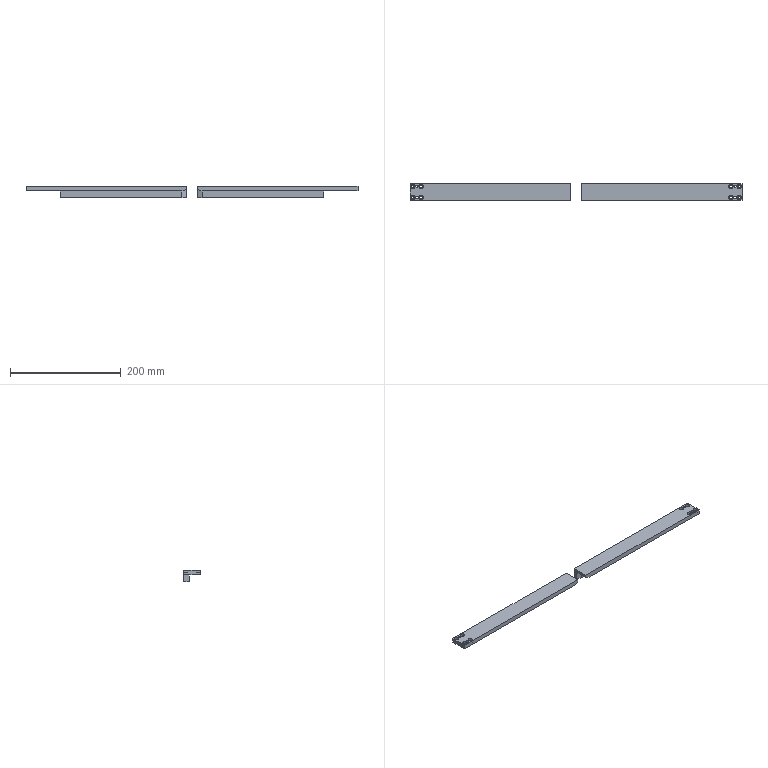NC program | NX | posted with a generic post | part box 600 x 30 x 20 mm
Lines 415 to 1233 of 3385:
(ZLEVEL_PROFILE_COPY_1_COPY_1 , TOOL : D3)
N792 T20 M6
N794 G54
N796 G17 G0 G90 X132.15 Y9.714 S7000 M3
N798 G43 Z30. H20
N800 Z1.
N802 G94 G1 X132.179 Y9.67 Z0.997 F1000.
N804 X132.383 Y9.555 Z0.985
N806 X132.617 Z0.973
N808 X132.821 Y9.67 Z0.96
N810 X132.927 Y9.829 Z0.95
N812 X132.951 Y10.089 Z0.937
N814 X132.83 Y10.321 Z0.923
N816 X132.671 Y10.427 Z0.913
N818 X132.595 Y10.45 Z0.909
N820 X132.405 Z0.899
N822 X132.179 Y10.33 Z0.885
N824 X132.073 Y10.171 Z0.875
N826 X132.04 Y10. Z0.866
N828 X132.073 Y9.829 Z0.857
N830 X132.179 Y9.67 Z0.847
N832 X132.383 Y9.555 Z0.835
N834 X132.617 Z0.823
N836 X132.821 Y9.67 Z0.81
N838 X132.927 Y9.829 Z0.8
N840 X132.951 Y10.089 Z0.787
N842 X132.83 Y10.321 Z0.773
N844 X132.671 Y10.427 Z0.763
N846 X132.595 Y10.45 Z0.759
N848 X132.405 Z0.749
N850 X132.179 Y10.33 Z0.735
N852 X132.073 Y10.171 Z0.725
N854 X132.04 Y10. Z0.716
N856 X132.073 Y9.829 Z0.707
N858 X132.179 Y9.67 Z0.697
N860 X132.383 Y9.555 Z0.685
N862 X132.617 Z0.673
N864 X132.821 Y9.67 Z0.66
N866 X132.927 Y9.829 Z0.65
N868 X132.951 Y10.089 Z0.637
N870 X132.83 Y10.321 Z0.623
N872 X132.671 Y10.427 Z0.613
N874 X132.595 Y10.45 Z0.609
N876 X132.405 Z0.599
N878 X132.179 Y10.33 Z0.585
N880 X132.073 Y10.171 Z0.575
N882 X132.04 Y10. Z0.566
N884 X132.073 Y9.829 Z0.557
N886 X132.179 Y9.67 Z0.547
N888 X132.383 Y9.555 Z0.535
N890 X132.617 Z0.523
N892 X132.821 Y9.67 Z0.51
N894 X132.927 Y9.829 Z0.5
N896 X132.951 Y10.089 Z0.487
N898 X132.83 Y10.321 Z0.473
N900 X132.671 Y10.427 Z0.463
N902 X132.595 Y10.45 Z0.459
N904 X132.405 Z0.449
N906 X132.179 Y10.33 Z0.435
N908 X132.073 Y10.171 Z0.425
N910 X132.04 Y10. Z0.416
N912 X132.073 Y9.829 Z0.407
N914 X132.179 Y9.67 Z0.397
N916 X132.383 Y9.555 Z0.385
N918 X132.617 Z0.373
N920 X132.821 Y9.67 Z0.36
N922 X132.927 Y9.829 Z0.35
N924 X132.951 Y10.089 Z0.337
N926 X132.83 Y10.321 Z0.323
N928 X132.671 Y10.427 Z0.313
N930 X132.595 Y10.45 Z0.309
N932 X132.405 Z0.299
N934 X132.179 Y10.33 Z0.285
N936 X132.073 Y10.171 Z0.275
N938 X132.04 Y10. Z0.266
N940 X132.073 Y9.829 Z0.257
N942 X132.179 Y9.67 Z0.247
N944 X132.383 Y9.555 Z0.235
N946 X132.617 Z0.223
N948 X132.821 Y9.67 Z0.21
N950 X132.927 Y9.829 Z0.2
N952 X132.951 Y10.089 Z0.187
N954 X132.83 Y10.321 Z0.173
N956 X132.671 Y10.427 Z0.163
N958 X132.595 Y10.45 Z0.159
N960 X132.405 Z0.149
N962 X132.179 Y10.33 Z0.135
N964 X132.073 Y10.171 Z0.125
N966 X132.04 Y10. Z0.116
N968 X132.073 Y9.829 Z0.107
N970 X132.179 Y9.67 Z0.097
N972 X132.383 Y9.555 Z0.085
N974 X132.617 Z0.073
N976 X132.821 Y9.67 Z0.06
N978 X132.927 Y9.829 Z0.05
N980 X132.951 Y10.089 Z0.037
N982 X132.83 Y10.321 Z0.023
N984 X132.671 Y10.427 Z0.013
N986 X132.595 Y10.45 Z0.009
N988 X132.405 Z-0.001
N990 X132.179 Y10.33 Z-0.015
N992 X132.073 Y10.171 Z-0.025
N994 X132.04 Y10. Z-0.034
N996 X132.073 Y9.829 Z-0.043
N998 X132.179 Y9.67 Z-0.053
N1000 X132.383 Y9.555 Z-0.065
N1002 X132.617 Z-0.077
N1004 X132.821 Y9.67 Z-0.09
N1006 X132.927 Y9.829 Z-0.1
N1008 X132.951 Y10.089 Z-0.113
N1010 X132.83 Y10.321 Z-0.127
N1012 X132.671 Y10.427 Z-0.137
N1014 X132.595 Y10.45 Z-0.141
N1016 X132.405 Z-0.151
N1018 X132.179 Y10.33 Z-0.165
N1020 X132.073 Y10.171 Z-0.175
N1022 X132.04 Y10. Z-0.184
N1024 X132.073 Y9.829 Z-0.193
N1026 X132.179 Y9.67 Z-0.203
N1028 X132.383 Y9.555 Z-0.215
N1030 X132.617 Z-0.227
N1032 X132.821 Y9.67 Z-0.24
N1034 X132.927 Y9.829 Z-0.25
N1036 X132.951 Y10.089 Z-0.263
N1038 X132.83 Y10.321 Z-0.277
N1040 X132.671 Y10.427 Z-0.287
N1042 X132.595 Y10.45 Z-0.291
N1044 X132.5 Z-0.296
N1046 G3 X132.05 Y10. R0.45 F1300.
N1048 X132.5 Y10.45 R-0.45
N1050 G1 X132.443 Y10.439 Z-0.305
N1052 X132.387 Y10.427 Z-0.313
N1054 X132.331 Y10.411 Z-0.321
N1056 X132.279 Y10.383 Z-0.329
N1058 X132.23 Y10.351 Z-0.337
N1060 X132.186 Y10.314 Z-0.346
N1062 X132.149 Y10.27 Z-0.354
N1064 X132.117 Y10.221 Z-0.362
N1066 X132.089 Y10.169 Z-0.37
N1068 X132.073 Y10.113 Z-0.379
N1070 X132.054 Y10.059 Z-0.387
N1072 X132.05 Y10. Z-0.395
N1074 X132.054 Y9.941 Z-0.403
N1076 X132.065 Y9.884 Z-0.412
N1078 X132.084 Y9.828 Z-0.42
N1080 X132.11 Y9.775 Z-0.428
N1082 X132.149 Y9.732 Z-0.436
N1084 X132.185 Y9.687 Z-0.444
N1086 X132.23 Y9.65 Z-0.453
N1088 X132.279 Y9.617 Z-0.461
N1090 X132.331 Y9.59 Z-0.469
N1092 X132.386 Y9.573 Z-0.477
N1094 X132.442 Y9.561 Z-0.486
N1096 X132.5 Y9.556 Z-0.494
N1098 X132.558 Y9.561 Z-0.502
N1100 X132.614 Y9.573 Z-0.51
N1102 X132.669 Y9.59 Z-0.519
N1104 X132.721 Y9.617 Z-0.527
N1106 X132.77 Y9.649 Z-0.535
N1108 X132.814 Y9.686 Z-0.543
N1110 X132.851 Y9.73 Z-0.551
N1112 X132.883 Y9.779 Z-0.56
N1114 X132.911 Y9.831 Z-0.568
N1116 X132.927 Y9.887 Z-0.576
N1118 X132.939 Y9.943 Z-0.584
N1120 X132.95 Y10. Z-0.593
N1122 G3 X132.5 Y10.45 R0.45
N1124 G1 X132.443 Y10.439 Z-0.601
N1126 X132.387 Y10.427 Z-0.609
N1128 X132.331 Y10.411 Z-0.617
N1130 X132.279 Y10.383 Z-0.626
N1132 X132.23 Y10.351 Z-0.634
N1134 X132.186 Y10.314 Z-0.642
N1136 X132.149 Y10.27 Z-0.65
N1138 X132.117 Y10.221 Z-0.658
N1140 X132.089 Y10.169 Z-0.667
N1142 X132.073 Y10.113 Z-0.675
N1144 X132.054 Y10.059 Z-0.683
N1146 X132.05 Y10. Z-0.691
N1148 X132.054 Y9.941 Z-0.7
N1150 X132.065 Y9.884 Z-0.708
N1152 X132.084 Y9.828 Z-0.716
N1154 X132.11 Y9.775 Z-0.724
N1156 X132.149 Y9.732 Z-0.733
N1158 X132.185 Y9.687 Z-0.741
N1160 X132.23 Y9.65 Z-0.749
N1162 X132.279 Y9.617 Z-0.757
N1164 X132.331 Y9.59 Z-0.765
N1166 X132.386 Y9.573 Z-0.774
N1168 X132.442 Y9.561 Z-0.782
N1170 X132.5 Y9.556 Z-0.79
N1172 X132.558 Y9.561 Z-0.798
N1174 X132.614 Y9.573 Z-0.807
N1176 X132.669 Y9.59 Z-0.815
N1178 X132.721 Y9.617 Z-0.823
N1180 X132.77 Y9.649 Z-0.831
N1182 X132.814 Y9.686 Z-0.84
N1184 X132.851 Y9.73 Z-0.848
N1186 X132.883 Y9.779 Z-0.856
N1188 X132.911 Y9.831 Z-0.864
N1190 X132.927 Y9.887 Z-0.872
N1192 X132.939 Y9.943 Z-0.881
N1194 X132.95 Y10. Z-0.889
N1196 G3 X132.5 Y10.45 R0.45
N1198 G1 X132.443 Y10.439 Z-0.897
N1200 X132.387 Y10.427 Z-0.905
N1202 X132.331 Y10.411 Z-0.914
N1204 X132.279 Y10.383 Z-0.922
N1206 X132.23 Y10.351 Z-0.93
N1208 X132.186 Y10.314 Z-0.938
N1210 X132.149 Y10.27 Z-0.947
N1212 X132.117 Y10.221 Z-0.955
N1214 X132.089 Y10.169 Z-0.963
N1216 X132.073 Y10.113 Z-0.971
N1218 X132.054 Y10.059 Z-0.979
N1220 X132.05 Y10. Z-0.988
N1222 X132.054 Y9.941 Z-0.996
N1224 X132.065 Y9.884 Z-1.004
N1226 X132.084 Y9.828 Z-1.012
N1228 X132.11 Y9.775 Z-1.021
N1230 X132.149 Y9.732 Z-1.029
N1232 X132.185 Y9.687 Z-1.037
N1234 X132.23 Y9.65 Z-1.045
N1236 X132.279 Y9.617 Z-1.053
N1238 X132.331 Y9.59 Z-1.062
N1240 X132.386 Y9.573 Z-1.07
N1242 X132.442 Y9.561 Z-1.078
N1244 X132.5 Y9.556 Z-1.086
N1246 X132.558 Y9.561 Z-1.095
N1248 X132.614 Y9.573 Z-1.103
N1250 X132.669 Y9.59 Z-1.111
N1252 X132.721 Y9.617 Z-1.119
N1254 X132.77 Y9.649 Z-1.128
N1256 X132.814 Y9.686 Z-1.136
N1258 X132.851 Y9.73 Z-1.144
N1260 X132.883 Y9.779 Z-1.152
N1262 X132.911 Y9.831 Z-1.16
N1264 X132.927 Y9.887 Z-1.169
N1266 X132.939 Y9.943 Z-1.177
N1268 X132.95 Y10. Z-1.185
N1270 G3 X132.5 Y10.45 R0.45
N1272 G1 X132.443 Y10.439 Z-1.193
N1274 X132.387 Y10.427 Z-1.202
N1276 X132.331 Y10.411 Z-1.21
N1278 X132.279 Y10.383 Z-1.218
N1280 X132.23 Y10.351 Z-1.226
N1282 X132.186 Y10.314 Z-1.235
N1284 X132.149 Y10.27 Z-1.243
N1286 X132.117 Y10.221 Z-1.251
N1288 X132.089 Y10.169 Z-1.259
N1290 X132.073 Y10.113 Z-1.267
N1292 X132.054 Y10.059 Z-1.276
N1294 X132.05 Y10. Z-1.284
N1296 X132.054 Y9.941 Z-1.292
N1298 X132.065 Y9.884 Z-1.3
N1300 X132.084 Y9.828 Z-1.309
N1302 X132.11 Y9.775 Z-1.317
N1304 X132.149 Y9.732 Z-1.325
N1306 X132.185 Y9.687 Z-1.333
N1308 X132.23 Y9.65 Z-1.342
N1310 X132.279 Y9.617 Z-1.35
N1312 X132.331 Y9.59 Z-1.358
N1314 X132.386 Y9.573 Z-1.366
N1316 X132.442 Y9.561 Z-1.374
N1318 X132.5 Y9.556 Z-1.383
N1320 X132.558 Y9.561 Z-1.391
N1322 X132.614 Y9.573 Z-1.399
N1324 X132.669 Y9.59 Z-1.407
N1326 X132.721 Y9.617 Z-1.416
N1328 X132.77 Y9.649 Z-1.424
N1330 X132.814 Y9.686 Z-1.432
N1332 X132.851 Y9.73 Z-1.44
N1334 X132.883 Y9.779 Z-1.449
N1336 X132.911 Y9.831 Z-1.457
N1338 X132.927 Y9.887 Z-1.465
N1340 X132.939 Y9.943 Z-1.473
N1342 X132.95 Y10. Z-1.481
N1344 G3 X132.5 Y10.45 R0.45
N1346 G1 X132.443 Y10.439 Z-1.49
N1348 X132.387 Y10.427 Z-1.498
N1350 X132.331 Y10.411 Z-1.506
N1352 X132.279 Y10.383 Z-1.514
N1354 X132.23 Y10.351 Z-1.523
N1356 X132.186 Y10.314 Z-1.531
N1358 X132.149 Y10.27 Z-1.539
N1360 X132.117 Y10.221 Z-1.547
N1362 X132.089 Y10.169 Z-1.556
N1364 X132.073 Y10.113 Z-1.564
N1366 X132.054 Y10.059 Z-1.572
N1368 X132.05 Y10. Z-1.58
N1370 X132.054 Y9.941 Z-1.588
N1372 X132.065 Y9.884 Z-1.597
N1374 X132.084 Y9.828 Z-1.605
N1376 X132.11 Y9.775 Z-1.613
N1378 X132.149 Y9.732 Z-1.621
N1380 X132.185 Y9.687 Z-1.63
N1382 X132.23 Y9.65 Z-1.638
N1384 X132.279 Y9.617 Z-1.646
N1386 X132.331 Y9.59 Z-1.654
N1388 X132.386 Y9.573 Z-1.663
N1390 X132.442 Y9.561 Z-1.671
N1392 X132.5 Y9.556 Z-1.679
N1394 X132.558 Y9.561 Z-1.687
N1396 X132.614 Y9.573 Z-1.695
N1398 X132.669 Y9.59 Z-1.704
N1400 X132.721 Y9.617 Z-1.712
N1402 X132.77 Y9.649 Z-1.72
N1404 X132.814 Y9.686 Z-1.728
N1406 X132.851 Y9.73 Z-1.737
N1408 X132.883 Y9.779 Z-1.745
N1410 X132.911 Y9.831 Z-1.753
N1412 X132.927 Y9.887 Z-1.761
N1414 X132.939 Y9.943 Z-1.77
N1416 X132.95 Y10. Z-1.778
N1418 G3 X132.5 Y10.45 R0.45
N1420 G1 X132.443 Y10.439 Z-1.786
N1422 X132.387 Y10.427 Z-1.794
N1424 X132.331 Y10.411 Z-1.802
N1426 X132.279 Y10.383 Z-1.811
N1428 X132.23 Y10.351 Z-1.819
N1430 X132.186 Y10.314 Z-1.827
N1432 X132.149 Y10.27 Z-1.835
N1434 X132.117 Y10.221 Z-1.844
N1436 X132.089 Y10.169 Z-1.852
N1438 X132.073 Y10.113 Z-1.86
N1440 X132.054 Y10.059 Z-1.868
N1442 X132.05 Y10. Z-1.877
N1444 X132.054 Y9.941 Z-1.885
N1446 X132.065 Y9.884 Z-1.893
N1448 X132.084 Y9.828 Z-1.901
N1450 X132.11 Y9.775 Z-1.909
N1452 X132.149 Y9.732 Z-1.918
N1454 X132.185 Y9.687 Z-1.926
N1456 X132.23 Y9.65 Z-1.934
N1458 X132.279 Y9.617 Z-1.942
N1460 X132.331 Y9.59 Z-1.951
N1462 X132.386 Y9.573 Z-1.959
N1464 X132.442 Y9.561 Z-1.967
N1466 X132.5 Y9.556 Z-1.975
N1468 X132.558 Y9.561 Z-1.984
N1470 X132.614 Y9.573 Z-1.992
N1472 X132.669 Y9.59 Z-2.
N1474 X132.721 Y9.617 Z-2.008
N1476 X132.77 Y9.649 Z-2.016
N1478 X132.814 Y9.686 Z-2.025
N1480 X132.851 Y9.73 Z-2.033
N1482 X132.883 Y9.779 Z-2.041
N1484 X132.911 Y9.831 Z-2.049
N1486 X132.927 Y9.887 Z-2.058
N1488 X132.939 Y9.943 Z-2.066
N1490 X132.95 Y10. Z-2.074
N1492 G3 X132.5 Y10.45 R0.45
N1494 G1 X132.443 Y10.439 Z-2.082
N1496 X132.387 Y10.427 Z-2.091
N1498 X132.331 Y10.411 Z-2.099
N1500 X132.279 Y10.383 Z-2.107
N1502 X132.23 Y10.351 Z-2.115
N1504 X132.186 Y10.314 Z-2.123
N1506 X132.149 Y10.27 Z-2.132
N1508 X132.117 Y10.221 Z-2.14
N1510 X132.089 Y10.169 Z-2.148
N1512 X132.073 Y10.113 Z-2.156
N1514 X132.054 Y10.059 Z-2.165
N1516 X132.05 Y10. Z-2.173
N1518 X132.054 Y9.941 Z-2.181
N1520 X132.065 Y9.884 Z-2.189
N1522 X132.084 Y9.828 Z-2.198
N1524 X132.11 Y9.775 Z-2.206
N1526 X132.149 Y9.732 Z-2.214
N1528 X132.185 Y9.687 Z-2.222
N1530 X132.23 Y9.65 Z-2.23
N1532 X132.279 Y9.617 Z-2.239
N1534 X132.331 Y9.59 Z-2.247
N1536 X132.386 Y9.573 Z-2.255
N1538 X132.442 Y9.561 Z-2.263
N1540 X132.5 Y9.556 Z-2.272
N1542 X132.558 Y9.561 Z-2.28
N1544 X132.614 Y9.573 Z-2.288
N1546 X132.669 Y9.59 Z-2.296
N1548 X132.721 Y9.617 Z-2.305
N1550 X132.77 Y9.649 Z-2.313
N1552 X132.814 Y9.686 Z-2.321
N1554 X132.851 Y9.73 Z-2.329
N1556 X132.883 Y9.779 Z-2.337
N1558 X132.911 Y9.831 Z-2.346
N1560 X132.927 Y9.887 Z-2.354
N1562 X132.939 Y9.943 Z-2.362
N1564 X132.95 Y10. Z-2.37
N1566 G3 X132.5 Y10.45 R0.45
N1568 G1 X132.443 Y10.439 Z-2.379
N1570 X132.387 Y10.427 Z-2.387
N1572 X132.331 Y10.411 Z-2.395
N1574 X132.279 Y10.383 Z-2.403
N1576 X132.23 Y10.351 Z-2.412
N1578 X132.186 Y10.314 Z-2.42
N1580 X132.149 Y10.27 Z-2.428
N1582 X132.117 Y10.221 Z-2.436
N1584 X132.089 Y10.169 Z-2.444
N1586 X132.073 Y10.113 Z-2.453
N1588 X132.054 Y10.059 Z-2.461
N1590 X132.05 Y10. Z-2.469
N1592 X132.054 Y9.941 Z-2.477
N1594 X132.065 Y9.884 Z-2.486
N1596 X132.084 Y9.828 Z-2.494
N1598 X132.11 Y9.775 Z-2.502
N1600 X132.149 Y9.732 Z-2.51
N1602 X132.185 Y9.687 Z-2.519
N1604 X132.23 Y9.65 Z-2.527
N1606 X132.279 Y9.617 Z-2.535
N1608 X132.331 Y9.59 Z-2.543
N1610 X132.386 Y9.573 Z-2.551
N1612 X132.442 Y9.561 Z-2.56
N1614 X132.5 Y9.556 Z-2.568
N1616 X132.558 Y9.561 Z-2.576
N1618 X132.614 Y9.573 Z-2.584
N1620 X132.669 Y9.59 Z-2.593
N1622 X132.721 Y9.617 Z-2.601
N1624 X132.77 Y9.649 Z-2.609
N1626 X132.814 Y9.686 Z-2.617
N1628 X132.851 Y9.73 Z-2.626
N1630 X132.883 Y9.779 Z-2.634
N1632 X132.911 Y9.831 Z-2.642
N1634 X132.927 Y9.887 Z-2.65
N1636 X132.939 Y9.943 Z-2.658
N1638 X132.95 Y10. Z-2.667
N1640 G3 X132.5 Y10.45 R0.45
N1642 G1 X132.443 Y10.439 Z-2.675
N1644 X132.387 Y10.427 Z-2.683
N1646 X132.331 Y10.411 Z-2.691
N1648 X132.279 Y10.383 Z-2.7
N1650 X132.23 Y10.351 Z-2.708
N1652 X132.186 Y10.314 Z-2.716
N1654 X132.149 Y10.27 Z-2.724
N1656 X132.117 Y10.221 Z-2.733
N1658 X132.089 Y10.169 Z-2.741
N1660 X132.073 Y10.113 Z-2.749
N1662 X132.054 Y10.059 Z-2.757
N1664 X132.05 Y10. Z-2.765
N1666 X132.054 Y9.941 Z-2.774
N1668 X132.065 Y9.884 Z-2.782
N1670 X132.084 Y9.828 Z-2.79
N1672 X132.11 Y9.775 Z-2.798
N1674 X132.149 Y9.732 Z-2.807
N1676 X132.185 Y9.687 Z-2.815
N1678 X132.23 Y9.65 Z-2.823
N1680 X132.279 Y9.617 Z-2.831
N1682 X132.331 Y9.59 Z-2.84
N1684 X132.386 Y9.573 Z-2.848
N1686 X132.442 Y9.561 Z-2.856
N1688 X132.5 Y9.556 Z-2.864
N1690 X132.558 Y9.561 Z-2.872
N1692 X132.614 Y9.573 Z-2.881
N1694 X132.669 Y9.59 Z-2.889
N1696 X132.721 Y9.617 Z-2.897
N1698 X132.77 Y9.649 Z-2.905
N1700 X132.814 Y9.686 Z-2.914
N1702 X132.851 Y9.73 Z-2.922
N1704 X132.883 Y9.779 Z-2.93
N1706 X132.911 Y9.831 Z-2.938
N1708 X132.927 Y9.887 Z-2.947
N1710 X132.939 Y9.943 Z-2.955
N1712 X132.95 Y10. Z-2.963
N1714 G3 X132.5 Y10.45 R0.45
N1716 G1 X132.443 Y10.439 Z-2.971
N1718 X132.387 Y10.427 Z-2.979
N1720 X132.331 Y10.411 Z-2.988
N1722 X132.279 Y10.383 Z-2.996
N1724 X132.23 Y10.351 Z-3.004
N1726 X132.186 Y10.314 Z-3.012
N1728 X132.149 Y10.27 Z-3.021
N1730 X132.117 Y10.221 Z-3.029
N1732 X132.089 Y10.169 Z-3.037
N1734 X132.073 Y10.113 Z-3.045
N1736 X132.054 Y10.059 Z-3.053
N1738 X132.05 Y10. Z-3.062
N1740 X132.054 Y9.941 Z-3.07
N1742 X132.065 Y9.884 Z-3.078
N1744 X132.084 Y9.828 Z-3.086
N1746 X132.11 Y9.775 Z-3.095
N1748 X132.149 Y9.732 Z-3.103
N1750 X132.185 Y9.687 Z-3.111
N1752 X132.23 Y9.65 Z-3.119
N1754 X132.279 Y9.617 Z-3.128
N1756 X132.331 Y9.589 Z-3.136
N1758 X132.386 Y9.573 Z-3.144
N1760 X132.442 Y9.561 Z-3.152
N1762 X132.5 Y9.556 Z-3.16
N1764 X132.558 Y9.561 Z-3.169
N1766 X132.614 Y9.573 Z-3.177
N1768 X132.669 Y9.589 Z-3.185
N1770 X132.721 Y9.617 Z-3.193
N1772 X132.77 Y9.649 Z-3.202
N1774 X132.814 Y9.686 Z-3.21
N1776 X132.851 Y9.73 Z-3.218
N1778 X132.883 Y9.779 Z-3.226
N1780 X132.911 Y9.831 Z-3.235
N1782 X132.927 Y9.887 Z-3.243
N1784 X132.939 Y9.943 Z-3.251
N1786 X132.95 Y10. Z-3.259
N1788 G3 X132.5 Y10.45 R0.45
N1790 G1 X132.443 Y10.439 Z-3.267
N1792 X132.387 Y10.427 Z-3.276
N1794 X132.331 Y10.411 Z-3.284
N1796 X132.279 Y10.383 Z-3.292
N1798 X132.23 Y10.351 Z-3.3
N1800 X132.186 Y10.314 Z-3.309
N1802 X132.149 Y10.27 Z-3.317
N1804 X132.117 Y10.221 Z-3.325
N1806 X132.089 Y10.169 Z-3.333
N1808 X132.073 Y10.113 Z-3.342
N1810 X132.054 Y10.059 Z-3.35
N1812 X132.05 Y10. Z-3.358
N1814 X132.054 Y9.941 Z-3.366
N1816 X132.065 Y9.884 Z-3.374
N1818 X132.084 Y9.828 Z-3.383
N1820 X132.11 Y9.775 Z-3.391
N1822 X132.149 Y9.732 Z-3.399
N1824 X132.185 Y9.687 Z-3.407
N1826 X132.23 Y9.65 Z-3.416
N1828 X132.279 Y9.617 Z-3.424
N1830 X132.331 Y9.589 Z-3.432
N1832 X132.386 Y9.573 Z-3.44
N1834 X132.442 Y9.561 Z-3.449
N1836 X132.5 Y9.556 Z-3.457
N1838 X132.558 Y9.561 Z-3.465
N1840 X132.614 Y9.573 Z-3.473
N1842 X132.669 Y9.589 Z-3.481
N1844 X132.721 Y9.617 Z-3.49
N1846 X132.77 Y9.649 Z-3.498
N1848 X132.814 Y9.686 Z-3.506
N1850 X132.851 Y9.73 Z-3.514
N1852 X132.883 Y9.779 Z-3.523
N1854 X132.911 Y9.831 Z-3.531
N1856 X132.927 Y9.887 Z-3.539
N1858 X132.939 Y9.943 Z-3.547
N1860 X132.95 Y10. Z-3.556
N1862 G3 X132.5 Y10.45 R0.45
N1864 G1 X132.443 Y10.439 Z-3.564
N1866 X132.387 Y10.427 Z-3.572
N1868 X132.331 Y10.411 Z-3.58
N1870 X132.279 Y10.383 Z-3.588
N1872 X132.23 Y10.351 Z-3.597
N1874 X132.186 Y10.314 Z-3.605
N1876 X132.149 Y10.27 Z-3.613
N1878 X132.117 Y10.221 Z-3.621
N1880 X132.089 Y10.169 Z-3.63
N1882 X132.073 Y10.113 Z-3.638
N1884 X132.054 Y10.059 Z-3.646
N1886 X132.05 Y10. Z-3.654
N1888 X132.054 Y9.941 Z-3.663
N1890 X132.065 Y9.884 Z-3.671
N1892 X132.084 Y9.828 Z-3.679
N1894 X132.11 Y9.775 Z-3.687
N1896 X132.149 Y9.732 Z-3.695
N1898 X132.185 Y9.687 Z-3.704
N1900 X132.23 Y9.65 Z-3.712
N1902 X132.279 Y9.617 Z-3.72
N1904 X132.331 Y9.589 Z-3.728
N1906 X132.386 Y9.573 Z-3.737
N1908 X132.442 Y9.561 Z-3.745
N1910 X132.5 Y9.556 Z-3.753
N1912 X132.558 Y9.561 Z-3.761
N1914 X132.614 Y9.573 Z-3.77
N1916 X132.669 Y9.589 Z-3.778
N1918 X132.721 Y9.617 Z-3.786
N1920 X132.77 Y9.649 Z-3.794
N1922 X132.814 Y9.686 Z-3.802
N1924 X132.851 Y9.73 Z-3.811
N1926 X132.883 Y9.779 Z-3.819
N1928 X132.911 Y9.831 Z-3.827
N1930 X132.927 Y9.887 Z-3.835
N1932 X132.939 Y9.943 Z-3.844
N1934 X132.95 Y10. Z-3.852
N1936 G3 X132.5 Y10.45 R0.45
N1938 G1 X132.443 Y10.439 Z-3.86
N1940 X132.387 Y10.427 Z-3.868
N1942 X132.331 Y10.411 Z-3.877
N1944 X132.279 Y10.383 Z-3.885
N1946 X132.23 Y10.351 Z-3.893
N1948 X132.186 Y10.314 Z-3.901
N1950 X132.149 Y10.27 Z-3.909
N1952 X132.117 Y10.221 Z-3.918
N1954 X132.089 Y10.169 Z-3.926
N1956 X132.073 Y10.113 Z-3.934
N1958 X132.054 Y10.059 Z-3.942
N1960 X132.05 Y10. Z-3.951
N1962 X132.054 Y9.941 Z-3.959
N1964 X132.065 Y9.884 Z-3.967
N1966 X132.084 Y9.828 Z-3.975
N1968 X132.11 Y9.775 Z-3.984
N1970 X132.149 Y9.732 Z-3.992
N1972 X132.185 Y9.687 Z-4.
N1974 X132.23 Y9.65 Z-4.008
N1976 X132.279 Y9.617 Z-4.016
N1978 X132.331 Y9.589 Z-4.025
N1980 X132.386 Y9.573 Z-4.033
N1982 X132.442 Y9.561 Z-4.041
N1984 X132.5 Y9.556 Z-4.049
N1986 X132.558 Y9.561 Z-4.058
N1988 X132.614 Y9.573 Z-4.066
N1990 X132.669 Y9.589 Z-4.074
N1992 X132.721 Y9.617 Z-4.082
N1994 X132.77 Y9.649 Z-4.091
N1996 X132.814 Y9.686 Z-4.099
N1998 X132.851 Y9.73 Z-4.107
N2000 X132.883 Y9.779 Z-4.115
N2002 X132.911 Y9.831 Z-4.123
N2004 X132.927 Y9.887 Z-4.132
N2006 X132.939 Y9.943 Z-4.14
N2008 X132.95 Y10. Z-4.148
N2010 G3 X132.5 Y10.45 R0.45
N2012 G1 X132.443 Y10.439 Z-4.156
N2014 X132.387 Y10.427 Z-4.165
N2016 X132.331 Y10.411 Z-4.173
N2018 X132.279 Y10.383 Z-4.181
N2020 X132.23 Y10.351 Z-4.189
N2022 X132.186 Y10.314 Z-4.198
N2024 X132.149 Y10.27 Z-4.206
N2026 X132.117 Y10.221 Z-4.214
N2028 X132.089 Y10.169 Z-4.222
N2030 X132.073 Y10.113 Z-4.23
N2032 X132.054 Y10.059 Z-4.239
N2034 X132.05 Y10. Z-4.247
N2036 X132.054 Y9.941 Z-4.255
N2038 X132.065 Y9.884 Z-4.263
N2040 X132.084 Y9.828 Z-4.272
N2042 X132.11 Y9.775 Z-4.28
N2044 X132.149 Y9.732 Z-4.288
N2046 X132.185 Y9.687 Z-4.296
N2048 X132.23 Y9.65 Z-4.305
N2050 X132.279 Y9.617 Z-4.313
N2052 X132.331 Y9.589 Z-4.321
N2054 X132.386 Y9.573 Z-4.329
N2056 X132.442 Y9.561 Z-4.337
N2058 X132.5 Y9.556 Z-4.346
N2060 X132.558 Y9.561 Z-4.354
N2062 X132.614 Y9.573 Z-4.362
N2064 X132.669 Y9.589 Z-4.37
N2066 X132.721 Y9.617 Z-4.379
N2068 X132.77 Y9.649 Z-4.387
N2070 X132.814 Y9.686 Z-4.395
N2072 X132.851 Y9.73 Z-4.403
N2074 X132.883 Y9.779 Z-4.412
N2076 X132.911 Y9.831 Z-4.42
N2078 X132.927 Y9.887 Z-4.428
N2080 X132.939 Y9.943 Z-4.436
N2082 X132.95 Y10. Z-4.444
N2084 G3 X132.5 Y10.45 R0.45
N2086 G1 X132.443 Y10.439 Z-4.453
N2088 X132.387 Y10.427 Z-4.461
N2090 X132.331 Y10.411 Z-4.469
N2092 X132.279 Y10.383 Z-4.477
N2094 X132.23 Y10.351 Z-4.486
N2096 X132.186 Y10.314 Z-4.494
N2098 X132.149 Y10.27 Z-4.502
N2100 X132.117 Y10.221 Z-4.51
N2102 X132.089 Y10.169 Z-4.519
N2104 X132.073 Y10.113 Z-4.527
N2106 X132.054 Y10.059 Z-4.535
N2108 X132.05 Y10. Z-4.543
N2110 X132.054 Y9.941 Z-4.551
N2112 X132.065 Y9.884 Z-4.56
N2114 X132.084 Y9.828 Z-4.568
N2116 X132.11 Y9.775 Z-4.576
N2118 X132.149 Y9.732 Z-4.584
N2120 X132.185 Y9.687 Z-4.593
N2122 X132.23 Y9.65 Z-4.601
N2124 X132.279 Y9.617 Z-4.609
N2126 X132.331 Y9.589 Z-4.617
N2128 X132.386 Y9.573 Z-4.626
N2130 X132.442 Y9.561 Z-4.634
N2132 X132.5 Y9.556 Z-4.642
N2134 X132.558 Y9.561 Z-4.65
N2136 X132.614 Y9.573 Z-4.658
N2138 X132.669 Y9.589 Z-4.667
N2140 X132.721 Y9.617 Z-4.675
N2142 X132.77 Y9.649 Z-4.683
N2144 X132.814 Y9.686 Z-4.691
N2146 X132.851 Y9.73 Z-4.7
N2148 X132.883 Y9.779 Z-4.708
N2150 X132.911 Y9.831 Z-4.716
N2152 X132.927 Y9.887 Z-4.724
N2154 X132.939 Y9.943 Z-4.733
N2156 X132.95 Y10. Z-4.741
N2158 G3 X132.5 Y10.45 R0.45
N2160 G1 X132.443 Y10.439 Z-4.749
N2162 X132.387 Y10.427 Z-4.757
N2164 X132.331 Y10.411 Z-4.765
N2166 X132.279 Y10.383 Z-4.774
N2168 X132.23 Y10.351 Z-4.782
N2170 X132.186 Y10.314 Z-4.79
N2172 X132.149 Y10.27 Z-4.798
N2174 X132.117 Y10.221 Z-4.807
N2176 X132.089 Y10.169 Z-4.815
N2178 X132.073 Y10.113 Z-4.823
N2180 X132.054 Y10.059 Z-4.831
N2182 X132.05 Y10. Z-4.84
N2184 X132.054 Y9.941 Z-4.848
N2186 X132.065 Y9.884 Z-4.856
N2188 X132.084 Y9.828 Z-4.864
N2190 X132.11 Y9.775 Z-4.872
N2192 X132.149 Y9.732 Z-4.881
N2194 X132.185 Y9.687 Z-4.889
N2196 X132.23 Y9.65 Z-4.897
N2198 X132.279 Y9.617 Z-4.905
N2200 X132.331 Y9.589 Z-4.914
N2202 X132.386 Y9.573 Z-4.922
N2204 X132.442 Y9.562 Z-4.93
N2206 X132.5 Y9.556 Z-4.938
N2208 X132.558 Y9.562 Z-4.947
N2210 X132.614 Y9.573 Z-4.955
N2212 X132.669 Y9.589 Z-4.963
N2214 X132.721 Y9.617 Z-4.971
N2216 X132.77 Y9.649 Z-4.979
N2218 X132.814 Y9.686 Z-4.988
N2220 X132.851 Y9.73 Z-4.996
N2222 X132.883 Y9.779 Z-5.004
N2224 X132.911 Y9.831 Z-5.012
N2226 X132.927 Y9.887 Z-5.021
N2228 X132.938 Y9.943 Z-5.029
N2230 X132.95 Y10. Z-5.037
N2232 G3 X132.5 Y10.45 R0.45
N2234 G1 X132.443 Y10.438 Z-5.045
N2236 X132.387 Y10.427 Z-5.053
N2238 X132.331 Y10.411 Z-5.062
N2240 X132.279 Y10.383 Z-5.07
N2242 X132.23 Y10.351 Z-5.078
N2244 X132.186 Y10.314 Z-5.086
N2246 X132.149 Y10.27 Z-5.095
N2248 X132.117 Y10.221 Z-5.103
N2250 X132.089 Y10.169 Z-5.111
N2252 X132.073 Y10.113 Z-5.119
N2254 X132.054 Y10.059 Z-5.128
N2256 X132.05 Y10. Z-5.136
N2258 X132.054 Y9.941 Z-5.144
N2260 X132.065 Y9.884 Z-5.152
N2262 X132.084 Y9.828 Z-5.16
N2264 X132.11 Y9.775 Z-5.169
N2266 X132.149 Y9.732 Z-5.177
N2268 X132.185 Y9.687 Z-5.185
N2270 X132.23 Y9.65 Z-5.193
N2272 X132.279 Y9.617 Z-5.202
N2274 X132.331 Y9.589 Z-5.21
N2276 X132.386 Y9.573 Z-5.218
N2278 X132.442 Y9.562 Z-5.226
N2280 X132.5 Y9.556 Z-5.235
N2282 X132.558 Y9.562 Z-5.243
N2284 X132.614 Y9.573 Z-5.251
N2286 X132.669 Y9.589 Z-5.259
N2288 X132.721 Y9.617 Z-5.267
N2290 X132.77 Y9.649 Z-5.276
N2292 X132.814 Y9.686 Z-5.284
N2294 X132.851 Y9.73 Z-5.292
N2296 X132.883 Y9.779 Z-5.3
N2298 X132.911 Y9.831 Z-5.309
N2300 X132.927 Y9.887 Z-5.317
N2302 X132.938 Y9.943 Z-5.325
N2304 X132.95 Y10. Z-5.333
N2306 G3 X132.5 Y10.45 R0.45
N2308 G1 X132.443 Y10.438 Z-5.342
N2310 X132.387 Y10.427 Z-5.35
N2312 X132.331 Y10.411 Z-5.358
N2314 X132.279 Y10.383 Z-5.366
N2316 X132.23 Y10.351 Z-5.374
N2318 X132.186 Y10.314 Z-5.383
N2320 X132.149 Y10.27 Z-5.391
N2322 X132.117 Y10.221 Z-5.399
N2324 X132.089 Y10.169 Z-5.407
N2326 X132.073 Y10.113 Z-5.416
N2328 X132.054 Y10.059 Z-5.424
N2330 X132.05 Y10. Z-5.432
N2332 X132.054 Y9.941 Z-5.44
N2334 X132.065 Y9.884 Z-5.449
N2336 X132.084 Y9.828 Z-5.457
N2338 X132.11 Y9.775 Z-5.465
N2340 X132.149 Y9.732 Z-5.473
N2342 X132.185 Y9.687 Z-5.481
N2344 X132.23 Y9.65 Z-5.49
N2346 X132.279 Y9.617 Z-5.498
N2348 X132.331 Y9.589 Z-5.506
N2350 X132.386 Y9.573 Z-5.514
N2352 X132.442 Y9.562 Z-5.523
N2354 X132.5 Y9.556 Z-5.531
N2356 X132.558 Y9.562 Z-5.539
N2358 X132.614 Y9.573 Z-5.547
N2360 X132.669 Y9.589 Z-5.556
N2362 X132.721 Y9.617 Z-5.564
N2364 X132.77 Y9.649 Z-5.572
N2366 X132.814 Y9.686 Z-5.58
N2368 X132.851 Y9.73 Z-5.588
N2370 X132.883 Y9.779 Z-5.597
N2372 X132.911 Y9.831 Z-5.605
N2374 X132.927 Y9.887 Z-5.613
N2376 X132.938 Y9.943 Z-5.621
N2378 X132.95 Y10. Z-5.63
N2380 G3 X132.5 Y10.45 R0.45
N2382 G1 X132.443 Y10.438 Z-5.638
N2384 X132.387 Y10.427 Z-5.646
N2386 X132.331 Y10.411 Z-5.654
N2388 X132.279 Y10.383 Z-5.663
N2390 X132.23 Y10.351 Z-5.671
N2392 X132.186 Y10.314 Z-5.679
N2394 X132.149 Y10.27 Z-5.687
N2396 X132.117 Y10.221 Z-5.695
N2398 X132.089 Y10.169 Z-5.704
N2400 X132.073 Y10.113 Z-5.712
N2402 X132.054 Y10.059 Z-5.72
N2404 X132.05 Y10. Z-5.728
N2406 X132.054 Y9.941 Z-5.737
N2408 X132.065 Y9.884 Z-5.745
N2410 X132.084 Y9.828 Z-5.753
N2412 X132.11 Y9.775 Z-5.761
N2414 X132.149 Y9.732 Z-5.77
N2416 X132.185 Y9.687 Z-5.778
N2418 X132.23 Y9.65 Z-5.786
N2420 X132.279 Y9.617 Z-5.794
N2422 X132.331 Y9.589 Z-5.802